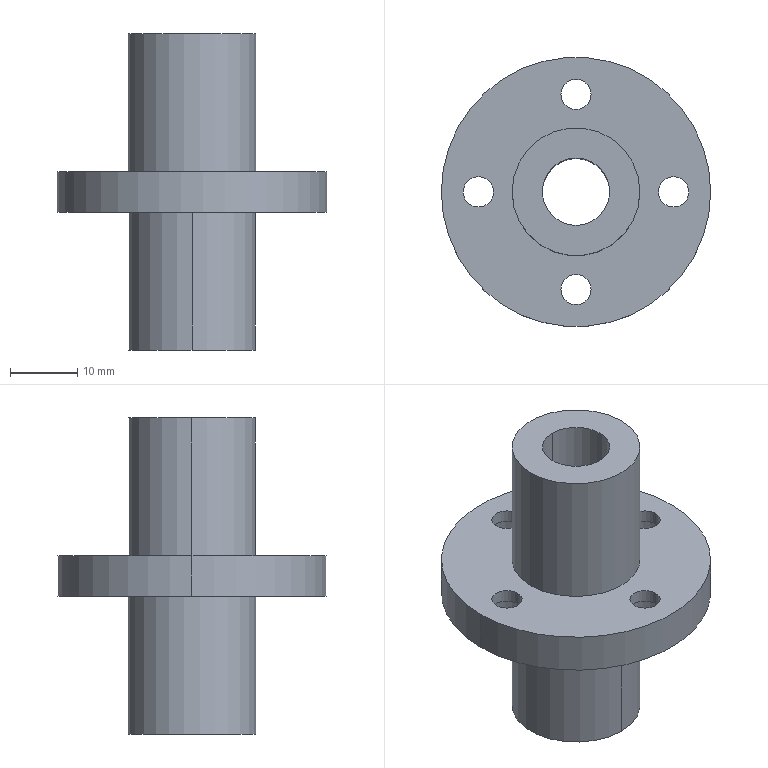Part | STEP file | Linear bearing LHMRD 10 | 1 solid | 32 faces | box 40 x 40 x 47 mm | volume 14628 mm3 | cylinder 24 | plane 8 | commonest cylinder face diameters 4.5 x8 7.5 x8 19 x4 10 x2 40 x2